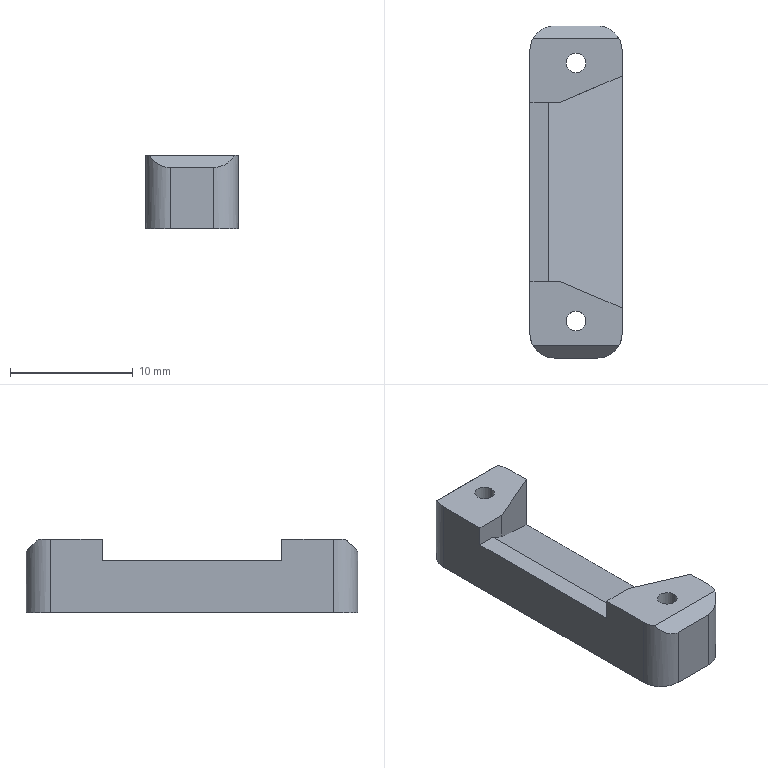NC program | NX | posted with a generic post | part box 7.5 x 27 x 6 mm
Whole program:
N10 G17 G21 G94 G90
(ADAPTIVE_MILLING_1 , TOOL : D4-ROUGH)
N12 T01 M6
N14 G54
N16 G17 G0 G90 X12.702 Y13.386 B0. C0. S6500 M3
N18 G43 Z30. H1
N20 Z3.1
N22 G94 G1 X12.568 Y13.318 Z2.163 F3000.
N24 X12.434 Y13.251 Z1.792
N26 X12.3 Y13.184 Z1.52
N28 X12.166 Y13.117 Z1.3
N30 X12.032 Y13.05 Z1.116
N32 X11.898 Y12.982 Z0.958
N34 X11.763 Y12.915 Z0.82
N36 X11.629 Y12.848 Z0.7
N38 X11.495 Y12.781 Z0.595
N40 X11.361 Y12.713 Z0.502
N42 X11.227 Y12.646 Z0.421
N44 X11.093 Y12.579 Z0.35
N46 X10.959 Y12.512 Z0.29
N48 X10.825 Y12.445 Z0.238
N50 X10.691 Y12.377 Z0.195
N52 X10.557 Y12.31 Z0.161
N54 X10.423 Y12.243 Z0.134
N56 X10.288 Y12.176 Z0.115
N58 X10.154 Y12.108 Z0.104
N60 X10.02 Y12.041 Z0.1
N62 G3 X9.113 Y11.566 R20.387
N64 X8.767 Y10.553 R1.973
N66 X8.603 Y6.309 R35.416
N68 G1 X8.6 Y3.813
N70 Y-22.387
N72 G2 X7.396 Y-24.238 R2.332
N74 X4.823 Y-24.975 R5.953
N76 X-0.573 Y-25.099 R65.244
N78 G1 X-6.07 Y-25.086
N80 G2 X-7.855 Y-23.694 R2.492
N82 X-8.508 Y-20.941 R6.93
N84 X-8.6 Y-14.693 R106.851
N86 G1 X-8.599 Y15.41
N88 G2 X-7.376 Y17.25 R2.35
N90 X-4.75 Y17.982 R6.095
N92 X0.547 Y18.099 R67.866
N94 X6.109 Y18.08 R172.888
N96 X7.896 Y16.614 R2.543
N98 X8.521 Y13.751 R7.442
N100 X8.388 Y10.805 R14.068
N102 G3 X8.203 Y5.459 R59.91
N104 G1 X8.2 Y-21.137
N106 G2 X6.52 Y-23.79 R3.048
N108 X3.592 Y-24.568 R7.339
N110 X-2.155 Y-24.699 R72.379
N112 X-5.035 Y-24.673 R46.417
N114 X-7.407 Y-22.798 R3.188
N116 X-8.105 Y-19.642 R8.525
N118 X-8.2 Y-13.594 R108.471
N120 G1 X-8.199 Y14.187
N122 G2 X-6.519 Y16.79 R3.054
N124 X-3.491 Y17.577 R7.485
N126 X2.906 Y17.7 R87.685
N128 X5.134 Y17.657 R19.021
N130 X7.407 Y15.797 R3.211
N132 X8.034 Y12.038 R7.772
N134 G3 X7.8 Y3.513 R118.528
N136 G1 X7.799 Y-20.187
N138 G2 X5.703 Y-23.412 R3.561
N140 X2.457 Y-24.18 R8.78
N142 X-4.089 Y-24.275 R79.881
N144 X-6.934 Y-22.158 R3.585
N146 X-7.688 Y-18.856 R9.05
N148 X-7.799 Y-12.059 R108.647
N150 G1 X-7.798 Y13.191
N152 G2 X-5.702 Y16.412 R3.558
N154 X-2.457 Y17.18 R8.777
N156 X4.089 Y17.275 R79.742
N158 X6.933 Y15.157 R3.578
N160 X7.547 Y11.943 R7.439
N162 G3 X7.405 Y4.758 R700.468
N164 G1 X7.4 Y2.363
N166 X7.399 Y-19.237
N168 G2 X4.955 Y-23.037 R3.954
N170 X1.601 Y-23.779 R9.825
N172 X-3.395 Y-23.859 R42.614
N174 X-6.522 Y-21.486 R3.921
N176 X-7.28 Y-18.087 R9.781
N178 X-7.399 Y-12.289 R88.668
N180 G1 Y12.111
N182 G2 X-4.881 Y16.071 R3.99
N184 X-1.324 Y16.799 R10.514
N186 X3.323 Y16.867 R49.073
N188 X6.605 Y14.218 R3.884
N190 X7.083 Y11.019 R9.534
N192 G3 X7. Y2.363 R881.676
N194 G1 X6.999 Y-18.437
N196 G2 X5.956 Y-21.482 R4.33
N198 X2.995 Y-23.07 R5.621
N200 X-1.379 Y-23.473 R21.876
N202 X-3.747 Y-23.204 R6.145
N204 X-6.228 Y-20.593 R4.408
N206 X-6.903 Y-16.97 R11.855
N208 X-6.999 Y-9.672 R144.169
N210 G1 X-6.998 Y11.428
N212 G2 X-5.962 Y14.476 R4.339
N214 X-2.995 Y16.07 R5.621
N216 X1.379 Y16.472 R21.92
N218 X3.748 Y16.203 R6.119
N220 X6.199 Y13.453 R4.211
N222 X6.645 Y9.945 R11.888
N224 G1 X6.601 Y2.313
N226 X6.599 Y-17.637
N228 G2 X5.935 Y-20.418 R5.069
N230 X3.061 Y-22.476 R5.08
N232 X-1.089 Y-23.04 R15.843
N234 X-3.925 Y-22.414 R4.879
N236 X-5.997 Y-19.489 R5.093
N238 X-6.541 Y-15.436 R16.189
N240 X-6.599 Y-9.287 R259.973
N242 G1 X-6.598 Y10.563
N244 G2 X-6.048 Y13.226 R5.333
N246 X-3.222 Y15.424 R4.92
N248 X0.869 Y16.032 R14.858
N250 X3.51 Y15.631 R5.42
N252 X5.744 Y12.874 R4.457
N254 X6.216 Y9.218 R12.893
N256 G1 X6.201 Y2.263
N258 X6.199 Y-16.937
N260 G2 X5.632 Y-19.699 R5.7
N262 X2.755 Y-21.981 R5.039
N264 X-1.782 Y-22.533 R11.422
N266 X-5.19 Y-19.94 R4.409
N268 X-6.052 Y-16.26 R10.521
N270 X-6.198 Y-9.963 R85.34
N272 G1 X-6.199 Y9.637
N274 G2 X-5.86 Y12.199 R7.018
N276 X-2.989 Y14.895 R4.789
N278 X1.782 Y15.531 R11.262
N280 X5.094 Y12.86 R4.201
N282 X5.767 Y9.292 R10.512
N284 X5.801 Y2.363 R184.469
N286 G1 X5.799 Y-16.237
N288 G2 X5.324 Y-18.973 R6.446
N290 X2.409 Y-21.504 R5.029
N292 X-1.42 Y-22.029 R8.317
N294 X-4.784 Y-19.386 R4.467
N296 X-5.64 Y-15.755 R10.677
N298 X-5.798 Y-9.459 R80.465
N300 G1 Y8.991
N302 G2 X-5.438 Y11.702 R7.452
N304 X-2.495 Y14.47 R4.931
N306 X1.33 Y15.036 R8.354
N308 X4.599 Y12.437 R4.218
N310 X5.331 Y8.932 R10.21
N312 X5.401 Y2.113 R128.734
N314 G1 X5.399 Y-15.537
N316 G2 X4.992 Y-18.289 R7.336
N318 X1.978 Y-21.062 R5.075
N320 X-1.307 Y-21.445 R5.924
N322 X-4.352 Y-18.889 R4.473
N324 X-5.241 Y-15.114 R10.877
N326 X-5.397 Y-8.868 R82.064
N328 G1 X-5.398 Y8.282
N330 G2 X-5.079 Y11.051 R8.515
N332 X-2.071 Y14.024 R4.987
N334 X1.109 Y14.466 R5.943
N336 X4.117 Y11.987 R4.203
N338 X4.905 Y8.443 R10.118
N340 X5.002 Y4.345 R69.716
N342 G1 X5.001 Y-14.587
N344 G2 X4.717 Y-17.412 R9.757
N346 X1.513 Y-20.629 R5.032
N348 X-2.601 Y-20.072 R4.125
N350 X-4.426 Y-17.028 R5.746
N352 X-4.944 Y-12.669 R19.444
N354 X-4.998 Y-6.069 R325.288
N356 G1 X-4.997 Y7.931
N358 G2 X-4.585 Y10.784 R7.76
N360 X-1.18 Y13.736 R5.151
N362 X3.445 Y11.877 R3.895
N364 X4.435 Y8.44 R8.515
N366 X4.601 Y2.494 R61.8
N368 G1 X4.599 Y-14.256
N370 G2 X4.228 Y-17.167 R8.666
N372 X0.111 Y-20.276 R4.633
N374 X-3.205 Y-18.349 R3.909
N376 X-4.329 Y-14.906 R8.431
N378 X-4.592 Y-9.166 R47.008
N380 G1 X-4.598 Y-5.866
N382 X-4.596 Y7.334
N384 G2 X-4.2 Y10.241 R8.286
N386 X-0.387 Y13.238 R4.599
N388 X2.948 Y11.391 R3.689
N390 X4.004 Y7.979 R8.125
N392 X4.199 Y2.536 R51.05
N394 G1 X4.201 Y0.336
N396 X4.199 Y-13.614
N398 G2 X3.858 Y-16.582 R9.556
N400 X1.1 Y-19.41 R4.254
N402 X-2.468 Y-18.169 R3.44
N404 X-3.819 Y-14.972 R6.899
N406 X-4.175 Y-10.14 R30.108
N408 G1 X-4.198 Y-5.04
N410 G2 X-4.178 Y7.559 R913.723
N412 X-3.315 Y10.706 R5.956
N414 X-0.696 Y12.453 R3.695
N416 X2.388 Y10.934 R3.402
N418 X3.544 Y7.705 R7.235
N420 X3.794 Y2.565 R39.546
N422 G1 X3.8 Y-0.735
N424 X3.799 Y-13.035
N426 G2 X3.499 Y-15.959 R10.48
N428 X1.679 Y-18.367 R3.869
N430 X-1.779 Y-17.753 R3.016
N432 X-3.323 Y-14.774 R5.835
N434 X-3.758 Y-10.303 R22.971
N436 X-3.772 Y7.146 R839.681
N438 X-2.907 Y10.236 R5.912
N440 X1.384 Y10.809 R2.796
N442 X2.942 Y7.997 R5.274
N444 X3.371 Y3.576 R21.155
N446 G1 X3.4 Y-1.924
N448 G2 X3.374 Y-13.624 R722.
N450 X2.698 Y-16.414 R6.026
N452 X-0.948 Y-17.223 R2.535
N454 X-2.705 Y-14.789 R4.528
N456 X-3.317 Y-10.795 R14.764
N458 X-3.398 Y-3.796 R184.941
N460 X-3.37 Y6.653 R585.728
N462 X-2.751 Y9.308 R6.036
N464 X0.583 Y10.139 R2.362
N466 X2.357 Y7.776 R4.219
N468 X2.929 Y4.031 R13.681
N470 X3. Y-2.718 R194.214
N472 X2.973 Y-13.118 R605.374
N474 X2.538 Y-15.36 R5.882
N476 X-0.302 Y-16.272 R2.141
N478 X-2.194 Y-14.166 R3.794
N480 X-2.881 Y-10.647 R11.231
N482 X-2.997 Y-3.45 R124.816
N484 X-2.967 Y6.2 R436.941
N486 X-2.585 Y8.201 R5.358
N488 X-0.078 Y9.046 R1.973
N490 X1.817 Y7.075 R3.505
N492 X2.487 Y3.808 R10.064
N494 X2.6 Y-3.889 R131.785
N496 X2.567 Y-12.739 R354.165
N498 X2.317 Y-14.106 R3.466
N500 X0.19 Y-14.874 R1.787
N502 X-1.775 Y-13. R3.276
N504 X-2.468 Y-9.835 R9.389
N506 X-2.597 Y-3.788 R89.6
N508 X-2.573 Y5.562 R596.131
N510 X-2.389 Y6.687 R2.711
N512 X-0.564 Y7.388 R1.616
N514 X1.397 Y5.651 R3.038
N516 X2.092 Y2.492 R8.789
N518 X2.2 Y-3.656 R102.072
N520 X2.174 Y-11.905 R349.945
N522 X1.172 Y-12.768 R1.209
N524 X-1.036 Y-11.803 R2.187
N526 X-2.003 Y-8.997 R5.951
N528 X-2.194 Y-4.003 R45.016
N530 G1 X-2.186 Y4.11
N532 G2 X-0.748 Y4.922 R1.488
N534 X1.377 Y3.058 R2.282
N536 X1.77 Y-0.713 R16.423
N538 G1 X1.813 Y-8.213
N540 X1.961 Y-9.231
N542 X1.95 Y-9.295
N544 X1.791 Y-9.654 Z0.15
N546 X1.618 Y-10.007 Z0.2
N548 X1.395 Y-10.461 F15000.
N550 G2 X1.066 Y-10.632 R0.403
N552 G1 X-0.139 Y-10.636
N554 X-1.345 Y-10.626
N556 G2 X-2.229 Y-10.077 R1.186
N558 G1 X-2.605 Y-9.468
N560 G2 X-2.614 Y-9.171 R0.41
N562 G1 X-2.458 Y-8.747
N564 X-2.188 Y-8.009 Z0.1 F3000.
N566 X-2.134 Y-7.862
N568 G3 X-1.827 Y-5.515 R7.954
N570 G1 X-1.805 Y-1.812
N572 G2 X-2.076 Y-0.341 R6.435
N574 G1 X-2.089 Y-0.192 Z0.104
N576 X-2.102 Y-0.042 Z0.115
N578 X-2.114 Y0.107 Z0.134
N580 X-2.127 Y0.257 Z0.161
N582 X-2.14 Y0.406 Z0.195
N584 X-2.153 Y0.556 Z0.238
N586 X-2.165 Y0.705 Z0.29
N588 X-2.178 Y0.855 Z0.35
N590 X-2.191 Y1.004 Z0.421
N592 X-2.203 Y1.153 Z0.502
N594 X-2.216 Y1.303 Z0.595
N596 X-2.229 Y1.452 Z0.7
N598 X-2.242 Y1.602 Z0.82
N600 X-2.254 Y1.751 Z0.958
N602 X-2.267 Y1.901 Z1.116
N604 X-2.28 Y2.05 Z1.3
N606 X-2.292 Y2.2 Z1.52
N608 X-2.305 Y2.349 Z1.792
N610 X-2.318 Y2.499 Z2.163
N612 X-2.331 Y2.648 Z3.1
N614 G0 Z30.
N616 M5
(FLOOR_FACING_3 , TOOL : D4-FINISH)
N618 T02 M6
N620 G54
N622 G17 G0 G90 X2.671 Y17.429 B0. C0. S5500 M3
N624 G43 Z30. H2
N626 Z2.
N628 G94 G1 Z0. F800.
N630 X2.698 Y15.386
N632 X3.107 Y-15.263
N634 G2 X1.75 Y-15.5 R4.
N636 G1 X0.507
N638 X0.093 Y15.5
N640 X-1.75
N642 G3 X-2.51 Y15.427 R4.
N644 G1 X-2.096 Y-15.485
N646 X-2.07 Y-17.491
N648 Z2.
N650 G0 Z30.
N652 M5
(PLANAR_MILL_5 , TOOL : D3点钻)
N654 T03 M6
N656 G54
N658 G17 G0 G90 X5.75 Y12.5 B0. C0. S3500 M3
N660 G43 Z30. H3
N662 Z1.
N664 G94 G1 Z-1. F800.
N666 G3 X4.75 Y11.5 R1.
N668 G1 Y-11.5
N670 G2 X1.75 Y-14.5 R3.
N672 G1 X-1.75
N674 G2 X-4.75 Y-11.5 R3.
N676 G1 Y11.5
N678 G2 X-1.75 Y14.5 R3.
N680 G1 X1.75
N682 G2 X4.75 Y11.5 R3.
N684 G3 X5.75 Y10.5 R1.
N686 G1 Z1.
N688 G0 Z30.
(DRILLING_1 , TOOL : D3点钻)
N690 X0. Y-10.5 S3000
N692 G81 G98 Z-1. F200. R3.
N694 Y10.5
N696 G80
N698 G0 X0. Y10.5 Z30.
N700 M5
N702 M2